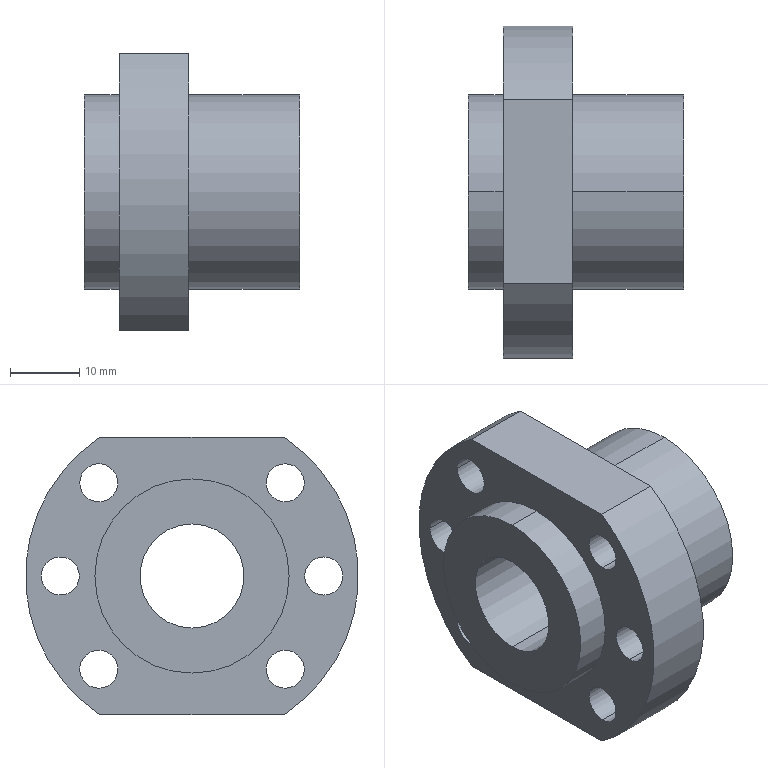Part | NX | features BREP 1 | 1 solid | 26 faces | box 31 x 48 x 40 mm | volume 22682 mm3 | cylinder 20 | plane 6 | commonest cylinder face diameters 5.5 x12 28 x4 15 x2 48 x2
STEP:
#1=CARTESIAN_POINT('',(-75.362,-50.269,-3.566));
#2=VERTEX_POINT('',#1);
#3=CARTESIAN_POINT('',(-44.362,-50.269,-3.566));
#4=VERTEX_POINT('',#3);
#5=CARTESIAN_POINT('',(-99.403,-50.269,-3.566));
#6=DIRECTION('',(1.,0.,0.));
#7=VECTOR('',#6,1000.);
#8=LINE('',#5,#7);
#9=EDGE_CURVE('',#2,#4,#8,.T.);
#10=ORIENTED_EDGE('',*,*,#9,.F.);
#11=CARTESIAN_POINT('',(-75.362,-50.269,-18.566));
#12=VERTEX_POINT('',#11);
#13=CARTESIAN_POINT('',(-75.362,-50.269,-11.066));
#14=DIRECTION('',(-1.,0.,0.));
#15=DIRECTION('',(0.,0.,-1.));
#16=AXIS2_PLACEMENT_3D('',#13,#14,#15);
#17=CIRCLE('',#16,7.5);
#18=EDGE_CURVE('',#2,#12,#17,.T.);
#19=ORIENTED_EDGE('',*,*,#18,.T.);
#20=CARTESIAN_POINT('',(-44.362,-50.269,-18.566));
#21=VERTEX_POINT('',#20);
#22=CARTESIAN_POINT('',(-99.403,-50.269,-18.566));
#23=DIRECTION('',(1.,0.,0.));
#24=VECTOR('',#23,1000.);
#25=LINE('',#22,#24);
#26=EDGE_CURVE('',#12,#21,#25,.T.);
#27=ORIENTED_EDGE('',*,*,#26,.T.);
#28=CARTESIAN_POINT('',(-44.362,-50.269,-11.066));
#29=DIRECTION('',(1.,0.,0.));
#30=DIRECTION('',(0.,0.,-1.));
#31=AXIS2_PLACEMENT_3D('',#28,#29,#30);
#32=CIRCLE('',#31,7.5);
#33=EDGE_CURVE('',#21,#4,#32,.T.);
#34=ORIENTED_EDGE('',*,*,#33,.T.);
#35=EDGE_LOOP('',(#10,#19,#27,#34));
#36=FACE_BOUND('',#35,.T.);
#37=CARTESIAN_POINT('',(-99.403,-50.269,-11.066));
#38=DIRECTION('',(1.,0.,0.));
#39=DIRECTION('',(0.,0.,-1.));
#40=AXIS2_PLACEMENT_3D('',#37,#38,#39);
#41=CYLINDRICAL_SURFACE('',#40,7.5);
#42=ADVANCED_FACE('',(#36),#41,.F.);
#43=CARTESIAN_POINT('',(-70.362,-69.269,-13.816));
#44=VERTEX_POINT('',#43);
#45=CARTESIAN_POINT('',(-60.362,-69.269,-13.816));
#46=VERTEX_POINT('',#45);
#47=CARTESIAN_POINT('',(-25.362,-69.269,-13.816));
#48=DIRECTION('',(-1.,0.,0.));
#49=VECTOR('',#48,1000.);
#50=LINE('',#47,#49);
#51=EDGE_CURVE('',#44,#46,#50,.F.);
#52=ORIENTED_EDGE('',*,*,#51,.T.);
#53=CARTESIAN_POINT('',(-60.362,-69.269,-8.316));
#54=VERTEX_POINT('',#53);
#55=CARTESIAN_POINT('',(-60.362,-69.269,-11.066));
#56=DIRECTION('',(1.,0.,0.));
#57=DIRECTION('',(0.,0.,1.));
#58=AXIS2_PLACEMENT_3D('',#55,#56,#57);
#59=CIRCLE('',#58,2.75);
#60=EDGE_CURVE('',#46,#54,#59,.T.);
#61=ORIENTED_EDGE('',*,*,#60,.T.);
#62=CARTESIAN_POINT('',(-70.362,-69.269,-8.316));
#63=VERTEX_POINT('',#62);
#64=CARTESIAN_POINT('',(-25.362,-69.269,-8.316));
#65=DIRECTION('',(-1.,0.,0.));
#66=VECTOR('',#65,1000.);
#67=LINE('',#64,#66);
#68=EDGE_CURVE('',#63,#54,#67,.F.);
#69=ORIENTED_EDGE('',*,*,#68,.F.);
#70=CARTESIAN_POINT('',(-70.362,-69.269,-11.066));
#71=DIRECTION('',(1.,0.,0.));
#72=DIRECTION('',(0.,0.,1.));
#73=AXIS2_PLACEMENT_3D('',#70,#71,#72);
#74=CIRCLE('',#73,2.75);
#75=EDGE_CURVE('',#44,#63,#74,.T.);
#76=ORIENTED_EDGE('',*,*,#75,.F.);
#77=EDGE_LOOP('',(#52,#61,#69,#76));
#78=FACE_BOUND('',#77,.T.);
#79=CARTESIAN_POINT('',(-25.362,-69.269,-11.066));
#80=DIRECTION('',(-1.,0.,0.));
#81=DIRECTION('',(0.,0.,1.));
#82=AXIS2_PLACEMENT_3D('',#79,#80,#81);
#83=CYLINDRICAL_SURFACE('',#82,2.75);
#84=ADVANCED_FACE('',(#78),#83,.F.);
#85=CARTESIAN_POINT('',(-60.362,-37.002,8.934));
#86=VERTEX_POINT('',#85);
#87=CARTESIAN_POINT('',(-60.362,-37.002,-31.066));
#88=VERTEX_POINT('',#87);
#89=CARTESIAN_POINT('',(-60.362,-50.269,-11.066));
#90=DIRECTION('',(-1.,0.,0.));
#91=DIRECTION('',(0.,0.,1.));
#92=AXIS2_PLACEMENT_3D('',#89,#90,#91);
#93=CIRCLE('',#92,24.);
#94=EDGE_CURVE('',#86,#88,#93,.T.);
#95=ORIENTED_EDGE('',*,*,#94,.T.);
#96=CARTESIAN_POINT('',(-70.362,-37.002,-31.066));
#97=VERTEX_POINT('',#96);
#98=CARTESIAN_POINT('',(-60.362,-37.002,-31.066));
#99=DIRECTION('',(1.,0.,0.));
#100=VECTOR('',#99,1000.);
#101=LINE('',#98,#100);
#102=EDGE_CURVE('',#97,#88,#101,.T.);
#103=ORIENTED_EDGE('',*,*,#102,.F.);
#104=CARTESIAN_POINT('',(-70.362,-37.002,8.934));
#105=VERTEX_POINT('',#104);
#106=CARTESIAN_POINT('',(-70.362,-50.269,-11.066));
#107=DIRECTION('',(-1.,0.,0.));
#108=DIRECTION('',(0.,0.,1.));
#109=AXIS2_PLACEMENT_3D('',#106,#107,#108);
#110=CIRCLE('',#109,24.);
#111=EDGE_CURVE('',#105,#97,#110,.T.);
#112=ORIENTED_EDGE('',*,*,#111,.F.);
#113=CARTESIAN_POINT('',(-60.362,-37.002,8.934));
#114=DIRECTION('',(-1.,0.,0.));
#115=VECTOR('',#114,1000.);
#116=LINE('',#113,#115);
#117=EDGE_CURVE('',#86,#105,#116,.T.);
#118=ORIENTED_EDGE('',*,*,#117,.F.);
#119=EDGE_LOOP('',(#95,#103,#112,#118));
#120=FACE_BOUND('',#119,.T.);
#121=CARTESIAN_POINT('',(-60.362,-50.269,-11.066));
#122=DIRECTION('',(-1.,0.,0.));
#123=DIRECTION('',(0.,0.,1.));
#124=AXIS2_PLACEMENT_3D('',#121,#122,#123);
#125=CYLINDRICAL_SURFACE('',#124,24.);
#126=ADVANCED_FACE('',(#120),#125,.T.);
#127=CARTESIAN_POINT('',(-60.362,-63.535,-31.066));
#128=VERTEX_POINT('',#127);
#129=CARTESIAN_POINT('',(-60.362,-50.269,-31.066));
#130=DIRECTION('',(0.,-1.,0.));
#131=VECTOR('',#130,1000.);
#132=LINE('',#129,#131);
#133=EDGE_CURVE('',#88,#128,#132,.T.);
#134=ORIENTED_EDGE('',*,*,#133,.T.);
#135=CARTESIAN_POINT('',(-70.362,-63.535,-31.066));
#136=VERTEX_POINT('',#135);
#137=CARTESIAN_POINT('',(-60.362,-63.535,-31.066));
#138=DIRECTION('',(1.,0.,0.));
#139=VECTOR('',#138,1000.);
#140=LINE('',#137,#139);
#141=EDGE_CURVE('',#136,#128,#140,.T.);
#142=ORIENTED_EDGE('',*,*,#141,.F.);
#143=CARTESIAN_POINT('',(-70.362,-50.269,-31.066));
#144=DIRECTION('',(0.,-1.,0.));
#145=VECTOR('',#144,1000.);
#146=LINE('',#143,#145);
#147=EDGE_CURVE('',#97,#136,#146,.T.);
#148=ORIENTED_EDGE('',*,*,#147,.F.);
#149=ORIENTED_EDGE('',*,*,#102,.T.);
#150=EDGE_LOOP('',(#134,#142,#148,#149));
#151=FACE_BOUND('',#150,.T.);
#152=CARTESIAN_POINT('',(-60.362,-37.002,-31.066));
#153=DIRECTION('',(0.,0.,-1.));
#154=DIRECTION('',(-1.,0.,0.));
#155=AXIS2_PLACEMENT_3D('',#152,#153,#154);
#156=PLANE('',#155);
#157=ADVANCED_FACE('',(#151),#156,.T.);
#158=CARTESIAN_POINT('',(-60.362,-63.535,8.934));
#159=VERTEX_POINT('',#158);
#160=CARTESIAN_POINT('',(-60.362,-50.269,-11.066));
#161=DIRECTION('',(-1.,0.,0.));
#162=DIRECTION('',(0.,0.,1.));
#163=AXIS2_PLACEMENT_3D('',#160,#161,#162);
#164=CIRCLE('',#163,24.);
#165=EDGE_CURVE('',#128,#159,#164,.T.);
#166=ORIENTED_EDGE('',*,*,#165,.T.);
#167=CARTESIAN_POINT('',(-70.362,-63.535,8.934));
#168=VERTEX_POINT('',#167);
#169=CARTESIAN_POINT('',(-60.362,-63.535,8.934));
#170=DIRECTION('',(1.,0.,0.));
#171=VECTOR('',#170,1000.);
#172=LINE('',#169,#171);
#173=EDGE_CURVE('',#168,#159,#172,.T.);
#174=ORIENTED_EDGE('',*,*,#173,.F.);
#175=CARTESIAN_POINT('',(-70.362,-50.269,-11.066));
#176=DIRECTION('',(-1.,0.,0.));
#177=DIRECTION('',(0.,0.,1.));
#178=AXIS2_PLACEMENT_3D('',#175,#176,#177);
#179=CIRCLE('',#178,24.);
#180=EDGE_CURVE('',#136,#168,#179,.T.);
#181=ORIENTED_EDGE('',*,*,#180,.F.);
#182=ORIENTED_EDGE('',*,*,#141,.T.);
#183=EDGE_LOOP('',(#166,#174,#181,#182));
#184=FACE_BOUND('',#183,.T.);
#185=CARTESIAN_POINT('',(-60.362,-50.269,-11.066));
#186=DIRECTION('',(-1.,0.,0.));
#187=DIRECTION('',(0.,0.,1.));
#188=AXIS2_PLACEMENT_3D('',#185,#186,#187);
#189=CYLINDRICAL_SURFACE('',#188,24.);
#190=ADVANCED_FACE('',(#184),#189,.T.);
#191=CARTESIAN_POINT('',(-60.362,-50.269,8.934));
#192=DIRECTION('',(0.,1.,0.));
#193=VECTOR('',#192,1000.);
#194=LINE('',#191,#193);
#195=EDGE_CURVE('',#159,#86,#194,.T.);
#196=ORIENTED_EDGE('',*,*,#195,.T.);
#197=ORIENTED_EDGE('',*,*,#117,.T.);
#198=CARTESIAN_POINT('',(-70.362,-50.269,8.934));
#199=DIRECTION('',(0.,1.,0.));
#200=VECTOR('',#199,1000.);
#201=LINE('',#198,#200);
#202=EDGE_CURVE('',#168,#105,#201,.T.);
#203=ORIENTED_EDGE('',*,*,#202,.F.);
#204=ORIENTED_EDGE('',*,*,#173,.T.);
#205=EDGE_LOOP('',(#196,#197,#203,#204));
#206=FACE_BOUND('',#205,.T.);
#207=CARTESIAN_POINT('',(-60.362,-63.535,8.934));
#208=DIRECTION('',(0.,0.,1.));
#209=DIRECTION('',(1.,0.,0.));
#210=AXIS2_PLACEMENT_3D('',#207,#208,#209);
#211=PLANE('',#210);
#212=ADVANCED_FACE('',(#206),#211,.T.);
#213=CARTESIAN_POINT('',(-60.362,-28.519,-11.066));
#214=VERTEX_POINT('',#213);
#215=CARTESIAN_POINT('',(-70.362,-28.519,-11.066));
#216=VERTEX_POINT('',#215);
#217=CARTESIAN_POINT('',(-25.362,-28.519,-11.066));
#218=DIRECTION('',(-1.,0.,0.));
#219=VECTOR('',#218,1000.);
#220=LINE('',#217,#219);
#221=EDGE_CURVE('',#214,#216,#220,.T.);
#222=ORIENTED_EDGE('',*,*,#221,.F.);
#223=CARTESIAN_POINT('',(-60.362,-34.019,-11.066));
#224=VERTEX_POINT('',#223);
#225=CARTESIAN_POINT('',(-60.362,-31.269,-11.066));
#226=DIRECTION('',(1.,0.,0.));
#227=DIRECTION('',(0.,-1.,0.));
#228=AXIS2_PLACEMENT_3D('',#225,#226,#227);
#229=CIRCLE('',#228,2.75);
#230=EDGE_CURVE('',#214,#224,#229,.T.);
#231=ORIENTED_EDGE('',*,*,#230,.T.);
#232=CARTESIAN_POINT('',(-70.362,-34.019,-11.066));
#233=VERTEX_POINT('',#232);
#234=CARTESIAN_POINT('',(-25.362,-34.019,-11.066));
#235=DIRECTION('',(-1.,0.,0.));
#236=VECTOR('',#235,1000.);
#237=LINE('',#234,#236);
#238=EDGE_CURVE('',#224,#233,#237,.T.);
#239=ORIENTED_EDGE('',*,*,#238,.T.);
#240=CARTESIAN_POINT('',(-70.362,-31.269,-11.066));
#241=DIRECTION('',(1.,0.,0.));
#242=DIRECTION('',(0.,-1.,0.));
#243=AXIS2_PLACEMENT_3D('',#240,#241,#242);
#244=CIRCLE('',#243,2.75);
#245=EDGE_CURVE('',#216,#233,#244,.T.);
#246=ORIENTED_EDGE('',*,*,#245,.F.);
#247=EDGE_LOOP('',(#222,#231,#239,#246));
#248=FACE_BOUND('',#247,.T.);
#249=CARTESIAN_POINT('',(-25.362,-31.269,-11.066));
#250=DIRECTION('',(-1.,0.,0.));
#251=DIRECTION('',(0.,-1.,0.));
#252=AXIS2_PLACEMENT_3D('',#249,#250,#251);
#253=CYLINDRICAL_SURFACE('',#252,2.75);
#254=ADVANCED_FACE('',(#248),#253,.F.);
#255=CARTESIAN_POINT('',(-60.362,-34.084,2.369));
#256=VERTEX_POINT('',#255);
#257=CARTESIAN_POINT('',(-70.362,-34.084,2.369));
#258=VERTEX_POINT('',#257);
#259=CARTESIAN_POINT('',(-25.362,-34.084,2.369));
#260=DIRECTION('',(-1.,0.,0.));
#261=VECTOR('',#260,1000.);
#262=LINE('',#259,#261);
#263=EDGE_CURVE('',#256,#258,#262,.T.);
#264=ORIENTED_EDGE('',*,*,#263,.F.);
#265=CARTESIAN_POINT('',(-60.362,-39.584,2.369));
#266=VERTEX_POINT('',#265);
#267=CARTESIAN_POINT('',(-60.362,-36.834,2.369));
#268=DIRECTION('',(1.,0.,0.));
#269=DIRECTION('',(0.,-1.,0.));
#270=AXIS2_PLACEMENT_3D('',#267,#268,#269);
#271=CIRCLE('',#270,2.75);
#272=EDGE_CURVE('',#256,#266,#271,.T.);
#273=ORIENTED_EDGE('',*,*,#272,.T.);
#274=CARTESIAN_POINT('',(-70.362,-39.584,2.369));
#275=VERTEX_POINT('',#274);
#276=CARTESIAN_POINT('',(-25.362,-39.584,2.369));
#277=DIRECTION('',(-1.,0.,0.));
#278=VECTOR('',#277,1000.);
#279=LINE('',#276,#278);
#280=EDGE_CURVE('',#266,#275,#279,.T.);
#281=ORIENTED_EDGE('',*,*,#280,.T.);
#282=CARTESIAN_POINT('',(-70.362,-36.834,2.369));
#283=DIRECTION('',(1.,0.,0.));
#284=DIRECTION('',(0.,-1.,0.));
#285=AXIS2_PLACEMENT_3D('',#282,#283,#284);
#286=CIRCLE('',#285,2.75);
#287=EDGE_CURVE('',#258,#275,#286,.T.);
#288=ORIENTED_EDGE('',*,*,#287,.F.);
#289=EDGE_LOOP('',(#264,#273,#281,#288));
#290=FACE_BOUND('',#289,.T.);
#291=CARTESIAN_POINT('',(-25.362,-36.834,2.369));
#292=DIRECTION('',(-1.,0.,0.));
#293=DIRECTION('',(0.,-1.,0.));
#294=AXIS2_PLACEMENT_3D('',#291,#292,#293);
#295=CYLINDRICAL_SURFACE('',#294,2.75);
#296=ADVANCED_FACE('',(#290),#295,.F.);
#297=CARTESIAN_POINT('',(-70.362,-36.834,-27.251));
#298=VERTEX_POINT('',#297);
#299=CARTESIAN_POINT('',(-60.362,-36.834,-27.251));
#300=VERTEX_POINT('',#299);
#301=CARTESIAN_POINT('',(-25.362,-36.834,-27.251));
#302=DIRECTION('',(-1.,0.,0.));
#303=VECTOR('',#302,1000.);
#304=LINE('',#301,#303);
#305=EDGE_CURVE('',#298,#300,#304,.F.);
#306=ORIENTED_EDGE('',*,*,#305,.T.);
#307=CARTESIAN_POINT('',(-60.362,-36.834,-21.751));
#308=VERTEX_POINT('',#307);
#309=CARTESIAN_POINT('',(-60.362,-36.834,-24.501));
#310=DIRECTION('',(1.,0.,0.));
#311=DIRECTION('',(0.,0.,1.));
#312=AXIS2_PLACEMENT_3D('',#309,#310,#311);
#313=CIRCLE('',#312,2.75);
#314=EDGE_CURVE('',#300,#308,#313,.T.);
#315=ORIENTED_EDGE('',*,*,#314,.T.);
#316=CARTESIAN_POINT('',(-70.362,-36.834,-21.751));
#317=VERTEX_POINT('',#316);
#318=CARTESIAN_POINT('',(-25.362,-36.834,-21.751));
#319=DIRECTION('',(-1.,0.,0.));
#320=VECTOR('',#319,1000.);
#321=LINE('',#318,#320);
#322=EDGE_CURVE('',#317,#308,#321,.F.);
#323=ORIENTED_EDGE('',*,*,#322,.F.);
#324=CARTESIAN_POINT('',(-70.362,-36.834,-24.501));
#325=DIRECTION('',(1.,0.,0.));
#326=DIRECTION('',(0.,0.,1.));
#327=AXIS2_PLACEMENT_3D('',#324,#325,#326);
#328=CIRCLE('',#327,2.75);
#329=EDGE_CURVE('',#298,#317,#328,.T.);
#330=ORIENTED_EDGE('',*,*,#329,.F.);
#331=EDGE_LOOP('',(#306,#315,#323,#330));
#332=FACE_BOUND('',#331,.T.);
#333=CARTESIAN_POINT('',(-25.362,-36.834,-24.501));
#334=DIRECTION('',(-1.,0.,0.));
#335=DIRECTION('',(0.,0.,1.));
#336=AXIS2_PLACEMENT_3D('',#333,#334,#335);
#337=CYLINDRICAL_SURFACE('',#336,2.75);
#338=ADVANCED_FACE('',(#332),#337,.F.);
#339=CARTESIAN_POINT('',(-70.362,-63.704,-27.251));
#340=VERTEX_POINT('',#339);
#341=CARTESIAN_POINT('',(-60.362,-63.704,-27.251));
#342=VERTEX_POINT('',#341);
#343=CARTESIAN_POINT('',(-25.362,-63.704,-27.251));
#344=DIRECTION('',(-1.,0.,0.));
#345=VECTOR('',#344,1000.);
#346=LINE('',#343,#345);
#347=EDGE_CURVE('',#340,#342,#346,.F.);
#348=ORIENTED_EDGE('',*,*,#347,.T.);
#349=CARTESIAN_POINT('',(-60.362,-63.704,-21.751));
#350=VERTEX_POINT('',#349);
#351=CARTESIAN_POINT('',(-60.362,-63.704,-24.501));
#352=DIRECTION('',(1.,0.,0.));
#353=DIRECTION('',(0.,0.,1.));
#354=AXIS2_PLACEMENT_3D('',#351,#352,#353);
#355=CIRCLE('',#354,2.75);
#356=EDGE_CURVE('',#342,#350,#355,.T.);
#357=ORIENTED_EDGE('',*,*,#356,.T.);
#358=CARTESIAN_POINT('',(-70.362,-63.704,-21.751));
#359=VERTEX_POINT('',#358);
#360=CARTESIAN_POINT('',(-25.362,-63.704,-21.751));
#361=DIRECTION('',(-1.,0.,0.));
#362=VECTOR('',#361,1000.);
#363=LINE('',#360,#362);
#364=EDGE_CURVE('',#359,#350,#363,.F.);
#365=ORIENTED_EDGE('',*,*,#364,.F.);
#366=CARTESIAN_POINT('',(-70.362,-63.704,-24.501));
#367=DIRECTION('',(1.,0.,0.));
#368=DIRECTION('',(0.,0.,1.));
#369=AXIS2_PLACEMENT_3D('',#366,#367,#368);
#370=CIRCLE('',#369,2.75);
#371=EDGE_CURVE('',#340,#359,#370,.T.);
#372=ORIENTED_EDGE('',*,*,#371,.F.);
#373=EDGE_LOOP('',(#348,#357,#365,#372));
#374=FACE_BOUND('',#373,.T.);
#375=CARTESIAN_POINT('',(-25.362,-63.704,-24.501));
#376=DIRECTION('',(-1.,0.,0.));
#377=DIRECTION('',(0.,0.,1.));
#378=AXIS2_PLACEMENT_3D('',#375,#376,#377);
#379=CYLINDRICAL_SURFACE('',#378,2.75);
#380=ADVANCED_FACE('',(#374),#379,.F.);
#381=CARTESIAN_POINT('',(-70.362,-63.704,-0.3809));
#382=VERTEX_POINT('',#381);
#383=CARTESIAN_POINT('',(-60.362,-63.704,-0.3809));
#384=VERTEX_POINT('',#383);
#385=CARTESIAN_POINT('',(-25.362,-63.704,-0.3809));
#386=DIRECTION('',(-1.,0.,0.));
#387=VECTOR('',#386,1000.);
#388=LINE('',#385,#387);
#389=EDGE_CURVE('',#382,#384,#388,.F.);
#390=ORIENTED_EDGE('',*,*,#389,.T.);
#391=CARTESIAN_POINT('',(-60.362,-63.704,5.119));
#392=VERTEX_POINT('',#391);
#393=CARTESIAN_POINT('',(-60.362,-63.704,2.369));
#394=DIRECTION('',(1.,0.,0.));
#395=DIRECTION('',(0.,0.,1.));
#396=AXIS2_PLACEMENT_3D('',#393,#394,#395);
#397=CIRCLE('',#396,2.75);
#398=EDGE_CURVE('',#384,#392,#397,.T.);
#399=ORIENTED_EDGE('',*,*,#398,.T.);
#400=CARTESIAN_POINT('',(-70.362,-63.704,5.119));
#401=VERTEX_POINT('',#400);
#402=CARTESIAN_POINT('',(-25.362,-63.704,5.119));
#403=DIRECTION('',(-1.,0.,0.));
#404=VECTOR('',#403,1000.);
#405=LINE('',#402,#404);
#406=EDGE_CURVE('',#401,#392,#405,.F.);
#407=ORIENTED_EDGE('',*,*,#406,.F.);
#408=CARTESIAN_POINT('',(-70.362,-63.704,2.369));
#409=DIRECTION('',(1.,0.,0.));
#410=DIRECTION('',(0.,0.,1.));
#411=AXIS2_PLACEMENT_3D('',#408,#409,#410);
#412=CIRCLE('',#411,2.75);
#413=EDGE_CURVE('',#382,#401,#412,.T.);
#414=ORIENTED_EDGE('',*,*,#413,.F.);
#415=EDGE_LOOP('',(#390,#399,#407,#414));
#416=FACE_BOUND('',#415,.T.);
#417=CARTESIAN_POINT('',(-25.362,-63.704,2.369));
#418=DIRECTION('',(-1.,0.,0.));
#419=DIRECTION('',(0.,0.,1.));
#420=AXIS2_PLACEMENT_3D('',#417,#418,#419);
#421=CYLINDRICAL_SURFACE('',#420,2.75);
#422=ADVANCED_FACE('',(#416),#421,.F.);
#423=CARTESIAN_POINT('',(-60.362,-69.269,-11.066));
#424=DIRECTION('',(1.,0.,0.));
#425=DIRECTION('',(0.,0.,1.));
#426=AXIS2_PLACEMENT_3D('',#423,#424,#425);
#427=CIRCLE('',#426,2.75);
#428=EDGE_CURVE('',#54,#46,#427,.T.);
#429=ORIENTED_EDGE('',*,*,#428,.F.);
#430=ORIENTED_EDGE('',*,*,#60,.F.);
#431=EDGE_LOOP('',(#429,#430));
#432=FACE_BOUND('',#431,.T.);
#433=CARTESIAN_POINT('',(-60.362,-50.269,2.934));
#434=VERTEX_POINT('',#433);
#435=CARTESIAN_POINT('',(-60.362,-50.269,-25.066));
#436=VERTEX_POINT('',#435);
#437=CARTESIAN_POINT('',(-60.362,-50.269,-11.066));
#438=DIRECTION('',(1.,0.,0.));
#439=DIRECTION('',(0.,0.,1.));
#440=AXIS2_PLACEMENT_3D('',#437,#438,#439);
#441=CIRCLE('',#440,14.);
#442=EDGE_CURVE('',#434,#436,#441,.T.);
#443=ORIENTED_EDGE('',*,*,#442,.F.);
#444=CARTESIAN_POINT('',(-60.362,-50.269,-11.066));
#445=DIRECTION('',(1.,0.,0.));
#446=DIRECTION('',(0.,0.,1.));
#447=AXIS2_PLACEMENT_3D('',#444,#445,#446);
#448=CIRCLE('',#447,14.);
#449=EDGE_CURVE('',#436,#434,#448,.T.);
#450=ORIENTED_EDGE('',*,*,#449,.F.);
#451=EDGE_LOOP('',(#443,#450));
#452=FACE_BOUND('',#451,.T.);
#453=ORIENTED_EDGE('',*,*,#195,.F.);
#454=ORIENTED_EDGE('',*,*,#165,.F.);
#455=ORIENTED_EDGE('',*,*,#133,.F.);
#456=ORIENTED_EDGE('',*,*,#94,.F.);
#457=EDGE_LOOP('',(#453,#454,#455,#456));
#458=FACE_BOUND('',#457,.T.);
#459=CARTESIAN_POINT('',(-60.362,-31.269,-11.066));
#460=DIRECTION('',(1.,0.,0.));
#461=DIRECTION('',(0.,-1.,0.));
#462=AXIS2_PLACEMENT_3D('',#459,#460,#461);
#463=CIRCLE('',#462,2.75);
#464=EDGE_CURVE('',#224,#214,#463,.T.);
#465=ORIENTED_EDGE('',*,*,#464,.F.);
#466=ORIENTED_EDGE('',*,*,#230,.F.);
#467=EDGE_LOOP('',(#465,#466));
#468=FACE_BOUND('',#467,.T.);
#469=CARTESIAN_POINT('',(-60.362,-36.834,2.369));
#470=DIRECTION('',(1.,0.,0.));
#471=DIRECTION('',(0.,-1.,0.));
#472=AXIS2_PLACEMENT_3D('',#469,#470,#471);
#473=CIRCLE('',#472,2.75);
#474=EDGE_CURVE('',#266,#256,#473,.T.);
#475=ORIENTED_EDGE('',*,*,#474,.F.);
#476=ORIENTED_EDGE('',*,*,#272,.F.);
#477=EDGE_LOOP('',(#475,#476));
#478=FACE_BOUND('',#477,.T.);
#479=CARTESIAN_POINT('',(-60.362,-36.834,-24.501));
#480=DIRECTION('',(1.,0.,0.));
#481=DIRECTION('',(0.,0.,1.));
#482=AXIS2_PLACEMENT_3D('',#479,#480,#481);
#483=CIRCLE('',#482,2.75);
#484=EDGE_CURVE('',#308,#300,#483,.T.);
#485=ORIENTED_EDGE('',*,*,#484,.F.);
#486=ORIENTED_EDGE('',*,*,#314,.F.);
#487=EDGE_LOOP('',(#485,#486));
#488=FACE_BOUND('',#487,.T.);
#489=CARTESIAN_POINT('',(-60.362,-63.704,-24.501));
#490=DIRECTION('',(1.,0.,0.));
#491=DIRECTION('',(0.,0.,1.));
#492=AXIS2_PLACEMENT_3D('',#489,#490,#491);
#493=CIRCLE('',#492,2.75);
#494=EDGE_CURVE('',#350,#342,#493,.T.);
#495=ORIENTED_EDGE('',*,*,#494,.F.);
#496=ORIENTED_EDGE('',*,*,#356,.F.);
#497=EDGE_LOOP('',(#495,#496));
#498=FACE_BOUND('',#497,.T.);
#499=CARTESIAN_POINT('',(-60.362,-63.704,2.369));
#500=DIRECTION('',(1.,0.,0.));
#501=DIRECTION('',(0.,0.,1.));
#502=AXIS2_PLACEMENT_3D('',#499,#500,#501);
#503=CIRCLE('',#502,2.75);
#504=EDGE_CURVE('',#392,#384,#503,.T.);
#505=ORIENTED_EDGE('',*,*,#504,.F.);
#506=ORIENTED_EDGE('',*,*,#398,.F.);
#507=EDGE_LOOP('',(#505,#506));
#508=FACE_BOUND('',#507,.T.);
#509=CARTESIAN_POINT('',(-60.362,-50.269,-11.066));
#510=DIRECTION('',(-1.,0.,0.));
#511=DIRECTION('',(0.,0.,1.));
#512=AXIS2_PLACEMENT_3D('',#509,#510,#511);
#513=PLANE('',#512);
#514=ADVANCED_FACE('',(#432,#452,#458,#468,#478,#488,#498,#508),#513,.F.);
#515=CARTESIAN_POINT('',(-70.362,-69.269,-11.066));
#516=DIRECTION('',(1.,0.,0.));
#517=DIRECTION('',(0.,0.,1.));
#518=AXIS2_PLACEMENT_3D('',#515,#516,#517);
#519=CIRCLE('',#518,2.75);
#520=EDGE_CURVE('',#63,#44,#519,.T.);
#521=ORIENTED_EDGE('',*,*,#520,.T.);
#522=ORIENTED_EDGE('',*,*,#75,.T.);
#523=EDGE_LOOP('',(#521,#522));
#524=FACE_BOUND('',#523,.T.);
#525=CARTESIAN_POINT('',(-70.362,-50.269,2.934));
#526=VERTEX_POINT('',#525);
#527=CARTESIAN_POINT('',(-70.362,-50.269,-25.066));
#528=VERTEX_POINT('',#527);
#529=CARTESIAN_POINT('',(-70.362,-50.269,-11.066));
#530=DIRECTION('',(-1.,0.,0.));
#531=DIRECTION('',(0.,0.,1.));
#532=AXIS2_PLACEMENT_3D('',#529,#530,#531);
#533=CIRCLE('',#532,14.);
#534=EDGE_CURVE('',#526,#528,#533,.T.);
#535=ORIENTED_EDGE('',*,*,#534,.F.);
#536=CARTESIAN_POINT('',(-70.362,-50.269,-11.066));
#537=DIRECTION('',(-1.,0.,0.));
#538=DIRECTION('',(0.,0.,1.));
#539=AXIS2_PLACEMENT_3D('',#536,#537,#538);
#540=CIRCLE('',#539,14.);
#541=EDGE_CURVE('',#528,#526,#540,.T.);
#542=ORIENTED_EDGE('',*,*,#541,.F.);
#543=EDGE_LOOP('',(#535,#542));
#544=FACE_BOUND('',#543,.T.);
#545=ORIENTED_EDGE('',*,*,#180,.T.);
#546=ORIENTED_EDGE('',*,*,#202,.T.);
#547=ORIENTED_EDGE('',*,*,#111,.T.);
#548=ORIENTED_EDGE('',*,*,#147,.T.);
#549=EDGE_LOOP('',(#545,#546,#547,#548));
#550=FACE_BOUND('',#549,.T.);
#551=CARTESIAN_POINT('',(-70.362,-31.269,-11.066));
#552=DIRECTION('',(1.,0.,0.));
#553=DIRECTION('',(0.,-1.,0.));
#554=AXIS2_PLACEMENT_3D('',#551,#552,#553);
#555=CIRCLE('',#554,2.75);
#556=EDGE_CURVE('',#233,#216,#555,.T.);
#557=ORIENTED_EDGE('',*,*,#556,.T.);
#558=ORIENTED_EDGE('',*,*,#245,.T.);
#559=EDGE_LOOP('',(#557,#558));
#560=FACE_BOUND('',#559,.T.);
#561=CARTESIAN_POINT('',(-70.362,-36.834,2.369));
#562=DIRECTION('',(1.,0.,0.));
#563=DIRECTION('',(0.,-1.,0.));
#564=AXIS2_PLACEMENT_3D('',#561,#562,#563);
#565=CIRCLE('',#564,2.75);
#566=EDGE_CURVE('',#275,#258,#565,.T.);
#567=ORIENTED_EDGE('',*,*,#566,.T.);
#568=ORIENTED_EDGE('',*,*,#287,.T.);
#569=EDGE_LOOP('',(#567,#568));
#570=FACE_BOUND('',#569,.T.);
#571=CARTESIAN_POINT('',(-70.362,-36.834,-24.501));
#572=DIRECTION('',(1.,0.,0.));
#573=DIRECTION('',(0.,0.,1.));
#574=AXIS2_PLACEMENT_3D('',#571,#572,#573);
#575=CIRCLE('',#574,2.75);
#576=EDGE_CURVE('',#317,#298,#575,.T.);
#577=ORIENTED_EDGE('',*,*,#576,.T.);
#578=ORIENTED_EDGE('',*,*,#329,.T.);
#579=EDGE_LOOP('',(#577,#578));
#580=FACE_BOUND('',#579,.T.);
#581=CARTESIAN_POINT('',(-70.362,-63.704,-24.501));
#582=DIRECTION('',(1.,0.,0.));
#583=DIRECTION('',(0.,0.,1.));
#584=AXIS2_PLACEMENT_3D('',#581,#582,#583);
#585=CIRCLE('',#584,2.75);
#586=EDGE_CURVE('',#359,#340,#585,.T.);
#587=ORIENTED_EDGE('',*,*,#586,.T.);
#588=ORIENTED_EDGE('',*,*,#371,.T.);
#589=EDGE_LOOP('',(#587,#588));
#590=FACE_BOUND('',#589,.T.);
#591=CARTESIAN_POINT('',(-70.362,-63.704,2.369));
#592=DIRECTION('',(1.,0.,0.));
#593=DIRECTION('',(0.,0.,1.));
#594=AXIS2_PLACEMENT_3D('',#591,#592,#593);
#595=CIRCLE('',#594,2.75);
#596=EDGE_CURVE('',#401,#382,#595,.T.);
#597=ORIENTED_EDGE('',*,*,#596,.T.);
#598=ORIENTED_EDGE('',*,*,#413,.T.);
#599=EDGE_LOOP('',(#597,#598));
#600=FACE_BOUND('',#599,.T.);
#601=CARTESIAN_POINT('',(-70.362,-50.269,-11.066));
#602=DIRECTION('',(-1.,0.,0.));
#603=DIRECTION('',(0.,0.,1.));
#604=AXIS2_PLACEMENT_3D('',#601,#602,#603);
#605=PLANE('',#604);
#606=ADVANCED_FACE('',(#524,#544,#550,#560,#570,#580,#590,#600),#605,.T.);
#607=CARTESIAN_POINT('',(-44.362,-50.269,-25.066));
#608=VERTEX_POINT('',#607);
#609=CARTESIAN_POINT('',(-56.862,-50.269,-25.066));
#610=DIRECTION('',(-1.,0.,0.));
#611=VECTOR('',#610,1000.);
#612=LINE('',#609,#611);
#613=EDGE_CURVE('',#436,#608,#612,.F.);
#614=ORIENTED_EDGE('',*,*,#613,.T.);
#615=CARTESIAN_POINT('',(-44.362,-50.269,2.934));
#616=VERTEX_POINT('',#615);
#617=CARTESIAN_POINT('',(-44.362,-50.269,-11.066));
#618=DIRECTION('',(-1.,0.,0.));
#619=DIRECTION('',(0.,0.,1.));
#620=AXIS2_PLACEMENT_3D('',#617,#618,#619);
#621=CIRCLE('',#620,14.);
#622=EDGE_CURVE('',#608,#616,#621,.T.);
#623=ORIENTED_EDGE('',*,*,#622,.T.);
#624=CARTESIAN_POINT('',(-56.862,-50.269,2.934));
#625=DIRECTION('',(-1.,0.,0.));
#626=VECTOR('',#625,1000.);
#627=LINE('',#624,#626);
#628=EDGE_CURVE('',#434,#616,#627,.F.);
#629=ORIENTED_EDGE('',*,*,#628,.F.);
#630=ORIENTED_EDGE('',*,*,#442,.T.);
#631=EDGE_LOOP('',(#614,#623,#629,#630));
#632=FACE_BOUND('',#631,.T.);
#633=CARTESIAN_POINT('',(-56.862,-50.269,-11.066));
#634=DIRECTION('',(-1.,0.,0.));
#635=DIRECTION('',(0.,0.,1.));
#636=AXIS2_PLACEMENT_3D('',#633,#634,#635);
#637=CYLINDRICAL_SURFACE('',#636,14.);
#638=ADVANCED_FACE('',(#632),#637,.T.);
#639=CARTESIAN_POINT('',(-75.362,-50.269,-25.066));
#640=VERTEX_POINT('',#639);
#641=CARTESIAN_POINT('',(-56.862,-50.269,-25.066));
#642=DIRECTION('',(-1.,0.,0.));
#643=VECTOR('',#642,1000.);
#644=LINE('',#641,#643);
#645=EDGE_CURVE('',#640,#528,#644,.F.);
#646=ORIENTED_EDGE('',*,*,#645,.T.);
#647=ORIENTED_EDGE('',*,*,#541,.T.);
#648=CARTESIAN_POINT('',(-75.362,-50.269,2.934));
#649=VERTEX_POINT('',#648);
#650=CARTESIAN_POINT('',(-56.862,-50.269,2.934));
#651=DIRECTION('',(-1.,0.,0.));
#652=VECTOR('',#651,1000.);
#653=LINE('',#650,#652);
#654=EDGE_CURVE('',#649,#526,#653,.F.);
#655=ORIENTED_EDGE('',*,*,#654,.F.);
#656=CARTESIAN_POINT('',(-75.362,-50.269,-11.066));
#657=DIRECTION('',(1.,0.,0.));
#658=DIRECTION('',(0.,0.,1.));
#659=AXIS2_PLACEMENT_3D('',#656,#657,#658);
#660=CIRCLE('',#659,14.);
#661=EDGE_CURVE('',#649,#640,#660,.T.);
#662=ORIENTED_EDGE('',*,*,#661,.T.);
#663=EDGE_LOOP('',(#646,#647,#655,#662));
#664=FACE_BOUND('',#663,.T.);
#665=CARTESIAN_POINT('',(-56.862,-50.269,-11.066));
#666=DIRECTION('',(-1.,0.,0.));
#667=DIRECTION('',(0.,0.,1.));
#668=AXIS2_PLACEMENT_3D('',#665,#666,#667);
#669=CYLINDRICAL_SURFACE('',#668,14.);
#670=ADVANCED_FACE('',(#664),#669,.T.);
#671=ORIENTED_EDGE('',*,*,#33,.F.);
#672=CARTESIAN_POINT('',(-44.362,-50.269,-11.066));
#673=DIRECTION('',(1.,0.,0.));
#674=DIRECTION('',(0.,0.,-1.));
#675=AXIS2_PLACEMENT_3D('',#672,#673,#674);
#676=CIRCLE('',#675,7.5);
#677=EDGE_CURVE('',#4,#21,#676,.T.);
#678=ORIENTED_EDGE('',*,*,#677,.F.);
#679=EDGE_LOOP('',(#671,#678));
#680=FACE_BOUND('',#679,.T.);
#681=CARTESIAN_POINT('',(-44.362,-50.269,-11.066));
#682=DIRECTION('',(-1.,0.,0.));
#683=DIRECTION('',(0.,0.,1.));
#684=AXIS2_PLACEMENT_3D('',#681,#682,#683);
#685=CIRCLE('',#684,14.);
#686=EDGE_CURVE('',#616,#608,#685,.T.);
#687=ORIENTED_EDGE('',*,*,#686,.F.);
#688=ORIENTED_EDGE('',*,*,#622,.F.);
#689=EDGE_LOOP('',(#687,#688));
#690=FACE_BOUND('',#689,.T.);
#691=CARTESIAN_POINT('',(-44.362,-38.519,-11.066));
#692=DIRECTION('',(-1.,0.,0.));
#693=DIRECTION('',(0.,0.,1.));
#694=AXIS2_PLACEMENT_3D('',#691,#692,#693);
#695=PLANE('',#694);
#696=ADVANCED_FACE('',(#680,#690),#695,.F.);
#697=CARTESIAN_POINT('',(-75.362,-50.269,-11.066));
#698=DIRECTION('',(-1.,0.,0.));
#699=DIRECTION('',(0.,0.,-1.));
#700=AXIS2_PLACEMENT_3D('',#697,#698,#699);
#701=CIRCLE('',#700,7.5);
#702=EDGE_CURVE('',#12,#2,#701,.T.);
#703=ORIENTED_EDGE('',*,*,#702,.F.);
#704=ORIENTED_EDGE('',*,*,#18,.F.);
#705=EDGE_LOOP('',(#703,#704));
#706=FACE_BOUND('',#705,.T.);
#707=ORIENTED_EDGE('',*,*,#661,.F.);
#708=CARTESIAN_POINT('',(-75.362,-50.269,-11.066));
#709=DIRECTION('',(1.,0.,0.));
#710=DIRECTION('',(0.,0.,1.));
#711=AXIS2_PLACEMENT_3D('',#708,#709,#710);
#712=CIRCLE('',#711,14.);
#713=EDGE_CURVE('',#640,#649,#712,.T.);
#714=ORIENTED_EDGE('',*,*,#713,.F.);
#715=EDGE_LOOP('',(#707,#714));
#716=FACE_BOUND('',#715,.T.);
#717=CARTESIAN_POINT('',(-75.362,-36.269,-11.066));
#718=DIRECTION('',(1.,0.,0.));
#719=DIRECTION('',(0.,0.,-1.));
#720=AXIS2_PLACEMENT_3D('',#717,#718,#719);
#721=PLANE('',#720);
#722=ADVANCED_FACE('',(#706,#716),#721,.F.);
#723=ORIENTED_EDGE('',*,*,#428,.T.);
#724=ORIENTED_EDGE('',*,*,#51,.F.);
#725=ORIENTED_EDGE('',*,*,#520,.F.);
#726=ORIENTED_EDGE('',*,*,#68,.T.);
#727=EDGE_LOOP('',(#723,#724,#725,#726));
#728=FACE_BOUND('',#727,.T.);
#729=CARTESIAN_POINT('',(-25.362,-69.269,-11.066));
#730=DIRECTION('',(-1.,0.,0.));
#731=DIRECTION('',(0.,0.,1.));
#732=AXIS2_PLACEMENT_3D('',#729,#730,#731);
#733=CYLINDRICAL_SURFACE('',#732,2.75);
#734=ADVANCED_FACE('',(#728),#733,.F.);
#735=ORIENTED_EDGE('',*,*,#464,.T.);
#736=ORIENTED_EDGE('',*,*,#221,.T.);
#737=ORIENTED_EDGE('',*,*,#556,.F.);
#738=ORIENTED_EDGE('',*,*,#238,.F.);
#739=EDGE_LOOP('',(#735,#736,#737,#738));
#740=FACE_BOUND('',#739,.T.);
#741=CARTESIAN_POINT('',(-25.362,-31.269,-11.066));
#742=DIRECTION('',(-1.,0.,0.));
#743=DIRECTION('',(0.,-1.,0.));
#744=AXIS2_PLACEMENT_3D('',#741,#742,#743);
#745=CYLINDRICAL_SURFACE('',#744,2.75);
#746=ADVANCED_FACE('',(#740),#745,.F.);
#747=ORIENTED_EDGE('',*,*,#474,.T.);
#748=ORIENTED_EDGE('',*,*,#263,.T.);
#749=ORIENTED_EDGE('',*,*,#566,.F.);
#750=ORIENTED_EDGE('',*,*,#280,.F.);
#751=EDGE_LOOP('',(#747,#748,#749,#750));
#752=FACE_BOUND('',#751,.T.);
#753=CARTESIAN_POINT('',(-25.362,-36.834,2.369));
#754=DIRECTION('',(-1.,0.,0.));
#755=DIRECTION('',(0.,-1.,0.));
#756=AXIS2_PLACEMENT_3D('',#753,#754,#755);
#757=CYLINDRICAL_SURFACE('',#756,2.75);
#758=ADVANCED_FACE('',(#752),#757,.F.);
#759=ORIENTED_EDGE('',*,*,#484,.T.);
#760=ORIENTED_EDGE('',*,*,#305,.F.);
#761=ORIENTED_EDGE('',*,*,#576,.F.);
#762=ORIENTED_EDGE('',*,*,#322,.T.);
#763=EDGE_LOOP('',(#759,#760,#761,#762));
#764=FACE_BOUND('',#763,.T.);
#765=CARTESIAN_POINT('',(-25.362,-36.834,-24.501));
#766=DIRECTION('',(-1.,0.,0.));
#767=DIRECTION('',(0.,0.,1.));
#768=AXIS2_PLACEMENT_3D('',#765,#766,#767);
#769=CYLINDRICAL_SURFACE('',#768,2.75);
#770=ADVANCED_FACE('',(#764),#769,.F.);
#771=ORIENTED_EDGE('',*,*,#494,.T.);
#772=ORIENTED_EDGE('',*,*,#347,.F.);
#773=ORIENTED_EDGE('',*,*,#586,.F.);
#774=ORIENTED_EDGE('',*,*,#364,.T.);
#775=EDGE_LOOP('',(#771,#772,#773,#774));
#776=FACE_BOUND('',#775,.T.);
#777=CARTESIAN_POINT('',(-25.362,-63.704,-24.501));
#778=DIRECTION('',(-1.,0.,0.));
#779=DIRECTION('',(0.,0.,1.));
#780=AXIS2_PLACEMENT_3D('',#777,#778,#779);
#781=CYLINDRICAL_SURFACE('',#780,2.75);
#782=ADVANCED_FACE('',(#776),#781,.F.);
#783=ORIENTED_EDGE('',*,*,#504,.T.);
#784=ORIENTED_EDGE('',*,*,#389,.F.);
#785=ORIENTED_EDGE('',*,*,#596,.F.);
#786=ORIENTED_EDGE('',*,*,#406,.T.);
#787=EDGE_LOOP('',(#783,#784,#785,#786));
#788=FACE_BOUND('',#787,.T.);
#789=CARTESIAN_POINT('',(-25.362,-63.704,2.369));
#790=DIRECTION('',(-1.,0.,0.));
#791=DIRECTION('',(0.,0.,1.));
#792=AXIS2_PLACEMENT_3D('',#789,#790,#791);
#793=CYLINDRICAL_SURFACE('',#792,2.75);
#794=ADVANCED_FACE('',(#788),#793,.F.);
#795=ORIENTED_EDGE('',*,*,#686,.T.);
#796=ORIENTED_EDGE('',*,*,#613,.F.);
#797=ORIENTED_EDGE('',*,*,#449,.T.);
#798=ORIENTED_EDGE('',*,*,#628,.T.);
#799=EDGE_LOOP('',(#795,#796,#797,#798));
#800=FACE_BOUND('',#799,.T.);
#801=CARTESIAN_POINT('',(-56.862,-50.269,-11.066));
#802=DIRECTION('',(-1.,0.,0.));
#803=DIRECTION('',(0.,0.,1.));
#804=AXIS2_PLACEMENT_3D('',#801,#802,#803);
#805=CYLINDRICAL_SURFACE('',#804,14.);
#806=ADVANCED_FACE('',(#800),#805,.T.);
#807=ORIENTED_EDGE('',*,*,#534,.T.);
#808=ORIENTED_EDGE('',*,*,#645,.F.);
#809=ORIENTED_EDGE('',*,*,#713,.T.);
#810=ORIENTED_EDGE('',*,*,#654,.T.);
#811=EDGE_LOOP('',(#807,#808,#809,#810));
#812=FACE_BOUND('',#811,.T.);
#813=CARTESIAN_POINT('',(-56.862,-50.269,-11.066));
#814=DIRECTION('',(-1.,0.,0.));
#815=DIRECTION('',(0.,0.,1.));
#816=AXIS2_PLACEMENT_3D('',#813,#814,#815);
#817=CYLINDRICAL_SURFACE('',#816,14.);
#818=ADVANCED_FACE('',(#812),#817,.T.);
#819=ORIENTED_EDGE('',*,*,#702,.T.);
#820=ORIENTED_EDGE('',*,*,#9,.T.);
#821=ORIENTED_EDGE('',*,*,#677,.T.);
#822=ORIENTED_EDGE('',*,*,#26,.F.);
#823=EDGE_LOOP('',(#819,#820,#821,#822));
#824=FACE_BOUND('',#823,.T.);
#825=CARTESIAN_POINT('',(-99.403,-50.269,-11.066));
#826=DIRECTION('',(1.,0.,0.));
#827=DIRECTION('',(0.,0.,-1.));
#828=AXIS2_PLACEMENT_3D('',#825,#826,#827);
#829=CYLINDRICAL_SURFACE('',#828,7.5);
#830=ADVANCED_FACE('',(#824),#829,.F.);
#831=CLOSED_SHELL('',(#42,#84,#126,#157,#190,#212,#254,#296,#338,#380,#422,#514,#606,#638,#670,#696,#722,#734,#746,#758,#770,#782,#794,#806,#818,#830));
#832=MANIFOLD_SOLID_BREP('',#831);
#833=(LENGTH_UNIT()NAMED_UNIT(*)SI_UNIT(.MILLI.,.METRE.));
#834=UNCERTAINTY_MEASURE_WITH_UNIT(LENGTH_MEASURE(0.00001),#833,'','');
#835=(NAMED_UNIT(*)PLANE_ANGLE_UNIT()SI_UNIT($,.RADIAN.));
#836=(NAMED_UNIT(*)SI_UNIT($,.STERADIAN.)SOLID_ANGLE_UNIT());
#837=(GEOMETRIC_REPRESENTATION_CONTEXT(3)GLOBAL_UNCERTAINTY_ASSIGNED_CONTEXT((#834))GLOBAL_UNIT_ASSIGNED_CONTEXT((#833,#835,#836))REPRESENTATION_CONTEXT('',''));
#838=ADVANCED_BREP_SHAPE_REPRESENTATION('',(#832),#837);